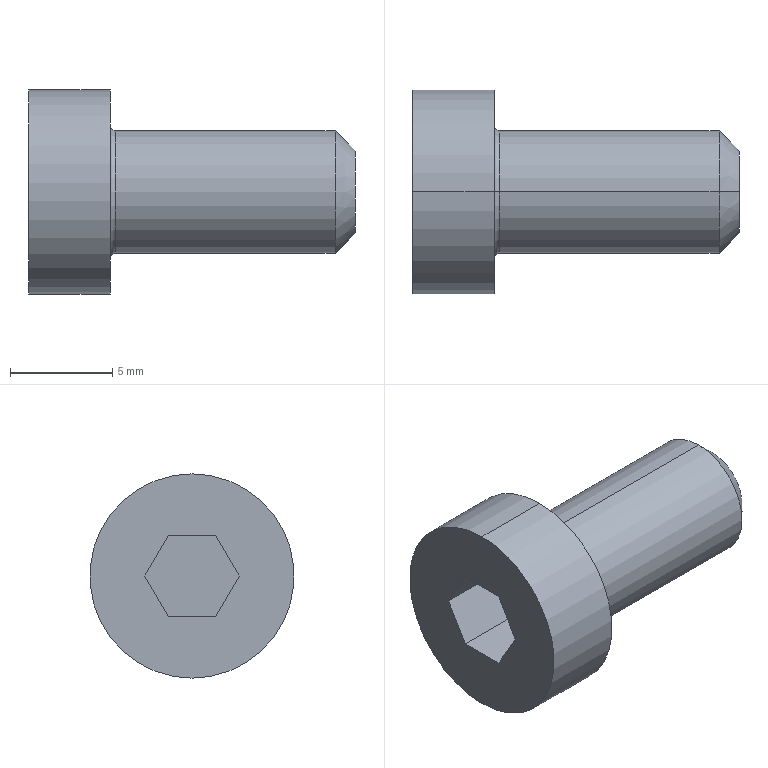Part | STEP file | CBSSTH6-12-24 | 1 solid | 18 faces | box 16 x 10 x 10 mm | volume 603.762 mm3 | plane 10 | cylinder 4 | torus 2 | cone 2 | commonest cylinder face diameters 6 x2 10 x2
STEP:
#1=CARTESIAN_POINT('',(0.,0.,0.));
#2=DIRECTION('',(0.,0.,1.));
#3=DIRECTION('',(1.,0.,0.));
#4=AXIS2_PLACEMENT_3D('',#1,#2,#3);
#5=CARTESIAN_POINT('',(0.,0.,5.));
#6=VERTEX_POINT('',#5);
#7=CARTESIAN_POINT('',(0.,0.,-5.));
#8=VERTEX_POINT('',#7);
#9=CARTESIAN_POINT('',(0.,0.,0.));
#10=DIRECTION('',(-1.,0.,0.));
#11=DIRECTION('',(0.,0.,1.));
#12=AXIS2_PLACEMENT_3D('',#9,#10,#11);
#13=CIRCLE('',#12,5.);
#14=CARTESIAN_POINT('',(-4.8,0.,0.));
#15=DIRECTION('',(-1.,0.,0.));
#16=DIRECTION('',(0.,0.,1.));
#17=AXIS2_PLACEMENT_3D('',#14,#15,#16);
#18=CYLINDRICAL_SURFACE('',#17,5.);
#19=CARTESIAN_POINT('',(0.,-4.8));
#20=DIRECTION('',(1.,0.));
#21=VECTOR('',#20,1.);
#22=LINE('',#19,#21);
#23=(GEOMETRIC_REPRESENTATION_CONTEXT(2)PARAMETRIC_REPRESENTATION_CONTEXT()REPRESENTATION_CONTEXT('',''));
#24=DEFINITIONAL_REPRESENTATION('',(#22),#23);
#25=PCURVE('',#18,#24);
#26=CARTESIAN_POINT('',(0.,-3.25,0.));
#27=DIRECTION('',(1.,0.,0.));
#28=DIRECTION('',(0.,0.,-1.));
#29=AXIS2_PLACEMENT_3D('',#26,#27,#28);
#30=PLANE('',#29);
#31=CARTESIAN_POINT('',(-5.,3.25));
#32=CARTESIAN_POINT('',(-5.,11.91));
#33=CARTESIAN_POINT('',(2.5,7.58));
#34=CARTESIAN_POINT('',(10.,3.25));
#35=CARTESIAN_POINT('',(2.5,-1.08));
#36=CARTESIAN_POINT('',(-5.,-5.41));
#37=CARTESIAN_POINT('',(-5.,3.25));
#38=(BOUNDED_CURVE()B_SPLINE_CURVE(2,(#31,#32,#33,#34,#35,#36,#37),.UNSPECIFIED.,.T.,.F.)B_SPLINE_CURVE_WITH_KNOTS((1,2,2,2,2,1),(-2.094,0.,2.094,4.189,6.283,8.378),.UNSPECIFIED.)CURVE()GEOMETRIC_REPRESENTATION_ITEM()RATIONAL_B_SPLINE_CURVE((1.,0.5,1.,0.5,1.,0.5,1.))REPRESENTATION_ITEM(''));
#39=(GEOMETRIC_REPRESENTATION_CONTEXT(2)PARAMETRIC_REPRESENTATION_CONTEXT()REPRESENTATION_CONTEXT('',''));
#40=DEFINITIONAL_REPRESENTATION('',(#38),#39);
#41=PCURVE('',#30,#40);
#42=SURFACE_CURVE('',#13,(#25,#41),.PCURVE_S1.);
#43=EDGE_CURVE('',#6,#8,#42,.T.);
#44=ORIENTED_EDGE('',*,*,#43,.T.);
#45=CARTESIAN_POINT('',(-4.,0.,-5.));
#46=VERTEX_POINT('',#45);
#47=CARTESIAN_POINT('',(-4.8,0.,-5.));
#48=DIRECTION('',(-1.,0.,0.));
#49=VECTOR('',#48,1.);
#50=LINE('',#47,#49);
#51=CARTESIAN_POINT('',(3.142,0.));
#52=DIRECTION('',(0.,1.));
#53=VECTOR('',#52,1.);
#54=LINE('',#51,#53);
#55=(GEOMETRIC_REPRESENTATION_CONTEXT(2)PARAMETRIC_REPRESENTATION_CONTEXT()REPRESENTATION_CONTEXT('',''));
#56=DEFINITIONAL_REPRESENTATION('',(#54),#55);
#57=PCURVE('',#18,#56);
#58=CARTESIAN_POINT('',(-4.8,0.,0.));
#59=DIRECTION('',(-1.,0.,0.));
#60=DIRECTION('',(0.,0.,1.));
#61=AXIS2_PLACEMENT_3D('',#58,#59,#60);
#62=CYLINDRICAL_SURFACE('',#61,5.);
#63=CARTESIAN_POINT('',(3.142,0.));
#64=DIRECTION('',(0.,1.));
#65=VECTOR('',#64,1.);
#66=LINE('',#63,#65);
#67=(GEOMETRIC_REPRESENTATION_CONTEXT(2)PARAMETRIC_REPRESENTATION_CONTEXT()REPRESENTATION_CONTEXT('',''));
#68=DEFINITIONAL_REPRESENTATION('',(#66),#67);
#69=PCURVE('',#62,#68);
#70=SURFACE_CURVE('',#50,(#57,#69),.PCURVE_S1.);
#71=EDGE_CURVE('',#8,#46,#70,.T.);
#72=ORIENTED_EDGE('',*,*,#71,.T.);
#73=CARTESIAN_POINT('',(-4.,0.,5.));
#74=VERTEX_POINT('',#73);
#75=CARTESIAN_POINT('',(-4.,0.,0.));
#76=DIRECTION('',(-1.,0.,0.));
#77=DIRECTION('',(0.,0.,1.));
#78=AXIS2_PLACEMENT_3D('',#75,#76,#77);
#79=CIRCLE('',#78,5.);
#80=CARTESIAN_POINT('',(0.,-0.8));
#81=DIRECTION('',(1.,0.));
#82=VECTOR('',#81,1.);
#83=LINE('',#80,#82);
#84=(GEOMETRIC_REPRESENTATION_CONTEXT(2)PARAMETRIC_REPRESENTATION_CONTEXT()REPRESENTATION_CONTEXT('',''));
#85=DEFINITIONAL_REPRESENTATION('',(#83),#84);
#86=PCURVE('',#18,#85);
#87=CARTESIAN_POINT('',(-4.,-5.,0.));
#88=DIRECTION('',(-1.,0.,0.));
#89=DIRECTION('',(0.,0.,1.));
#90=AXIS2_PLACEMENT_3D('',#87,#88,#89);
#91=PLANE('',#90);
#92=CARTESIAN_POINT('',(0.,5.));
#93=DIRECTION('',(1.,0.));
#94=AXIS2_PLACEMENT_2D('',#92,#93);
#95=CIRCLE('',#94,5.);
#96=(GEOMETRIC_REPRESENTATION_CONTEXT(2)PARAMETRIC_REPRESENTATION_CONTEXT()REPRESENTATION_CONTEXT('',''));
#97=DEFINITIONAL_REPRESENTATION('',(#95),#96);
#98=PCURVE('',#91,#97);
#99=SURFACE_CURVE('',#79,(#86,#98),.PCURVE_S1.);
#100=EDGE_CURVE('',#74,#46,#99,.T.);
#101=ORIENTED_EDGE('',*,*,#100,.F.);
#102=CARTESIAN_POINT('',(-4.8,0.,5.));
#103=DIRECTION('',(-1.,0.,0.));
#104=VECTOR('',#103,1.);
#105=LINE('',#102,#104);
#106=CARTESIAN_POINT('',(0.,0.));
#107=DIRECTION('',(0.,1.));
#108=VECTOR('',#107,1.);
#109=LINE('',#106,#108);
#110=(GEOMETRIC_REPRESENTATION_CONTEXT(2)PARAMETRIC_REPRESENTATION_CONTEXT()REPRESENTATION_CONTEXT('',''));
#111=DEFINITIONAL_REPRESENTATION('',(#109),#110);
#112=PCURVE('',#18,#111);
#113=CARTESIAN_POINT('',(6.283,0.));
#114=DIRECTION('',(0.,1.));
#115=VECTOR('',#114,1.);
#116=LINE('',#113,#115);
#117=(GEOMETRIC_REPRESENTATION_CONTEXT(2)PARAMETRIC_REPRESENTATION_CONTEXT()REPRESENTATION_CONTEXT('',''));
#118=DEFINITIONAL_REPRESENTATION('',(#116),#117);
#119=PCURVE('',#62,#118);
#120=SURFACE_CURVE('',#105,(#112,#119),.PCURVE_S1.);
#121=EDGE_CURVE('',#6,#74,#120,.T.);
#122=ORIENTED_EDGE('',*,*,#121,.F.);
#123=EDGE_LOOP('',(#44,#72,#101,#122));
#124=FACE_BOUND('',#123,.T.);
#125=ADVANCED_FACE('',(#124),#18,.T.);
#126=CARTESIAN_POINT('',(0.,0.,3.25));
#127=VERTEX_POINT('',#126);
#128=CARTESIAN_POINT('',(0.25,0.,3.));
#129=VERTEX_POINT('',#128);
#130=CARTESIAN_POINT('',(0.25,0.,3.25));
#131=DIRECTION('',(0.,-1.,0.));
#132=DIRECTION('',(0.,0.,-1.));
#133=AXIS2_PLACEMENT_3D('',#130,#131,#132);
#134=CIRCLE('',#133,0.25);
#135=CARTESIAN_POINT('',(0.25,0.,0.));
#136=DIRECTION('',(-1.,0.,0.));
#137=DIRECTION('',(0.,0.,1.));
#138=AXIS2_PLACEMENT_3D('',#135,#136,#137);
#139=TOROIDAL_SURFACE('',#138,3.25,0.25);
#140=CARTESIAN_POINT('',(6.283,-3.142));
#141=DIRECTION('',(0.,1.));
#142=VECTOR('',#141,1.);
#143=LINE('',#140,#142);
#144=(GEOMETRIC_REPRESENTATION_CONTEXT(2)PARAMETRIC_REPRESENTATION_CONTEXT()REPRESENTATION_CONTEXT('',''));
#145=DEFINITIONAL_REPRESENTATION('',(#143),#144);
#146=PCURVE('',#139,#145);
#147=CARTESIAN_POINT('',(0.25,0.,0.));
#148=DIRECTION('',(-1.,0.,0.));
#149=DIRECTION('',(0.,0.,1.));
#150=AXIS2_PLACEMENT_3D('',#147,#148,#149);
#151=TOROIDAL_SURFACE('',#150,3.25,0.25);
#152=CARTESIAN_POINT('',(0.,-3.142));
#153=DIRECTION('',(0.,1.));
#154=VECTOR('',#153,1.);
#155=LINE('',#152,#154);
#156=(GEOMETRIC_REPRESENTATION_CONTEXT(2)PARAMETRIC_REPRESENTATION_CONTEXT()REPRESENTATION_CONTEXT('',''));
#157=DEFINITIONAL_REPRESENTATION('',(#155),#156);
#158=PCURVE('',#151,#157);
#159=SURFACE_CURVE('',#134,(#146,#158),.PCURVE_S1.);
#160=EDGE_CURVE('',#127,#129,#159,.T.);
#161=ORIENTED_EDGE('',*,*,#160,.T.);
#162=CARTESIAN_POINT('',(0.25,0.,-3.));
#163=VERTEX_POINT('',#162);
#164=CARTESIAN_POINT('',(0.25,0.,0.));
#165=DIRECTION('',(-1.,0.,0.));
#166=DIRECTION('',(0.,0.,1.));
#167=AXIS2_PLACEMENT_3D('',#164,#165,#166);
#168=CIRCLE('',#167,3.);
#169=CARTESIAN_POINT('',(0.,3.142));
#170=DIRECTION('',(1.,0.));
#171=VECTOR('',#170,1.);
#172=LINE('',#169,#171);
#173=(GEOMETRIC_REPRESENTATION_CONTEXT(2)PARAMETRIC_REPRESENTATION_CONTEXT()REPRESENTATION_CONTEXT('',''));
#174=DEFINITIONAL_REPRESENTATION('',(#172),#173);
#175=PCURVE('',#139,#174);
#176=CARTESIAN_POINT('',(-4.8,0.,0.));
#177=DIRECTION('',(-1.,0.,0.));
#178=DIRECTION('',(0.,0.,1.));
#179=AXIS2_PLACEMENT_3D('',#176,#177,#178);
#180=CYLINDRICAL_SURFACE('',#179,3.);
#181=CARTESIAN_POINT('',(0.,-5.05));
#182=DIRECTION('',(1.,0.));
#183=VECTOR('',#182,1.);
#184=LINE('',#181,#183);
#185=(GEOMETRIC_REPRESENTATION_CONTEXT(2)PARAMETRIC_REPRESENTATION_CONTEXT()REPRESENTATION_CONTEXT('',''));
#186=DEFINITIONAL_REPRESENTATION('',(#184),#185);
#187=PCURVE('',#180,#186);
#188=SURFACE_CURVE('',#168,(#175,#187),.PCURVE_S1.);
#189=EDGE_CURVE('',#163,#129,#188,.T.);
#190=ORIENTED_EDGE('',*,*,#189,.F.);
#191=CARTESIAN_POINT('',(0.,0.,-3.25));
#192=VERTEX_POINT('',#191);
#193=CARTESIAN_POINT('',(0.25,0.,-3.25));
#194=DIRECTION('',(0.,1.,0.));
#195=DIRECTION('',(0.,0.,1.));
#196=AXIS2_PLACEMENT_3D('',#193,#194,#195);
#197=CIRCLE('',#196,0.25);
#198=CARTESIAN_POINT('',(3.142,-3.142));
#199=DIRECTION('',(0.,1.));
#200=VECTOR('',#199,1.);
#201=LINE('',#198,#200);
#202=(GEOMETRIC_REPRESENTATION_CONTEXT(2)PARAMETRIC_REPRESENTATION_CONTEXT()REPRESENTATION_CONTEXT('',''));
#203=DEFINITIONAL_REPRESENTATION('',(#201),#202);
#204=PCURVE('',#139,#203);
#205=CARTESIAN_POINT('',(3.142,-3.142));
#206=DIRECTION('',(0.,1.));
#207=VECTOR('',#206,1.);
#208=LINE('',#205,#207);
#209=(GEOMETRIC_REPRESENTATION_CONTEXT(2)PARAMETRIC_REPRESENTATION_CONTEXT()REPRESENTATION_CONTEXT('',''));
#210=DEFINITIONAL_REPRESENTATION('',(#208),#209);
#211=PCURVE('',#151,#210);
#212=SURFACE_CURVE('',#197,(#204,#211),.PCURVE_S1.);
#213=EDGE_CURVE('',#192,#163,#212,.T.);
#214=ORIENTED_EDGE('',*,*,#213,.F.);
#215=CARTESIAN_POINT('',(0.,0.,0.));
#216=DIRECTION('',(-1.,0.,0.));
#217=DIRECTION('',(0.,0.,1.));
#218=AXIS2_PLACEMENT_3D('',#215,#216,#217);
#219=CIRCLE('',#218,3.25);
#220=CARTESIAN_POINT('',(0.,1.571));
#221=DIRECTION('',(1.,0.));
#222=VECTOR('',#221,1.);
#223=LINE('',#220,#222);
#224=(GEOMETRIC_REPRESENTATION_CONTEXT(2)PARAMETRIC_REPRESENTATION_CONTEXT()REPRESENTATION_CONTEXT('',''));
#225=DEFINITIONAL_REPRESENTATION('',(#223),#224);
#226=PCURVE('',#139,#225);
#227=CARTESIAN_POINT('',(-3.25,3.25));
#228=CARTESIAN_POINT('',(-3.25,8.879));
#229=CARTESIAN_POINT('',(1.625,6.065));
#230=CARTESIAN_POINT('',(6.5,3.25));
#231=CARTESIAN_POINT('',(1.625,0.4354));
#232=CARTESIAN_POINT('',(-3.25,-2.379));
#233=CARTESIAN_POINT('',(-3.25,3.25));
#234=(BOUNDED_CURVE()B_SPLINE_CURVE(2,(#227,#228,#229,#230,#231,#232,#233),.UNSPECIFIED.,.T.,.F.)B_SPLINE_CURVE_WITH_KNOTS((1,2,2,2,2,1),(-2.094,0.,2.094,4.189,6.283,8.378),.UNSPECIFIED.)CURVE()GEOMETRIC_REPRESENTATION_ITEM()RATIONAL_B_SPLINE_CURVE((1.,0.5,1.,0.5,1.,0.5,1.))REPRESENTATION_ITEM(''));
#235=(GEOMETRIC_REPRESENTATION_CONTEXT(2)PARAMETRIC_REPRESENTATION_CONTEXT()REPRESENTATION_CONTEXT('',''));
#236=DEFINITIONAL_REPRESENTATION('',(#234),#235);
#237=PCURVE('',#30,#236);
#238=SURFACE_CURVE('',#219,(#226,#237),.PCURVE_S1.);
#239=EDGE_CURVE('',#192,#127,#238,.T.);
#240=ORIENTED_EDGE('',*,*,#239,.T.);
#241=EDGE_LOOP('',(#161,#190,#214,#240));
#242=FACE_BOUND('',#241,.F.);
#243=ADVANCED_FACE('',(#242),#139,.F.);
#244=CARTESIAN_POINT('',(11.,0.,3.));
#245=VERTEX_POINT('',#244);
#246=CARTESIAN_POINT('',(11.,0.,-3.));
#247=VERTEX_POINT('',#246);
#248=CARTESIAN_POINT('',(11.,0.,0.));
#249=DIRECTION('',(-1.,0.,0.));
#250=DIRECTION('',(0.,0.,1.));
#251=AXIS2_PLACEMENT_3D('',#248,#249,#250);
#252=CIRCLE('',#251,3.);
#253=CARTESIAN_POINT('',(-4.8,0.,0.));
#254=DIRECTION('',(-1.,0.,0.));
#255=DIRECTION('',(0.,0.,1.));
#256=AXIS2_PLACEMENT_3D('',#253,#254,#255);
#257=CYLINDRICAL_SURFACE('',#256,3.);
#258=CARTESIAN_POINT('',(0.,-15.8));
#259=DIRECTION('',(1.,0.));
#260=VECTOR('',#259,1.);
#261=LINE('',#258,#260);
#262=(GEOMETRIC_REPRESENTATION_CONTEXT(2)PARAMETRIC_REPRESENTATION_CONTEXT()REPRESENTATION_CONTEXT('',''));
#263=DEFINITIONAL_REPRESENTATION('',(#261),#262);
#264=PCURVE('',#257,#263);
#265=CARTESIAN_POINT('',(11.,0.,0.));
#266=DIRECTION('',(-1.,0.,0.));
#267=DIRECTION('',(0.,0.,1.));
#268=AXIS2_PLACEMENT_3D('',#265,#266,#267);
#269=CONICAL_SURFACE('',#268,3.,0.7854);
#270=CARTESIAN_POINT('',(0.,0.));
#271=DIRECTION('',(1.,0.));
#272=VECTOR('',#271,1.);
#273=LINE('',#270,#272);
#274=(GEOMETRIC_REPRESENTATION_CONTEXT(2)PARAMETRIC_REPRESENTATION_CONTEXT()REPRESENTATION_CONTEXT('',''));
#275=DEFINITIONAL_REPRESENTATION('',(#273),#274);
#276=PCURVE('',#269,#275);
#277=SURFACE_CURVE('',#252,(#264,#276),.PCURVE_S1.);
#278=EDGE_CURVE('',#245,#247,#277,.T.);
#279=ORIENTED_EDGE('',*,*,#278,.T.);
#280=CARTESIAN_POINT('',(-4.8,0.,-3.));
#281=DIRECTION('',(-1.,0.,0.));
#282=VECTOR('',#281,1.);
#283=LINE('',#280,#282);
#284=CARTESIAN_POINT('',(3.142,0.));
#285=DIRECTION('',(0.,1.));
#286=VECTOR('',#285,1.);
#287=LINE('',#284,#286);
#288=(GEOMETRIC_REPRESENTATION_CONTEXT(2)PARAMETRIC_REPRESENTATION_CONTEXT()REPRESENTATION_CONTEXT('',''));
#289=DEFINITIONAL_REPRESENTATION('',(#287),#288);
#290=PCURVE('',#257,#289);
#291=CARTESIAN_POINT('',(3.142,0.));
#292=DIRECTION('',(0.,1.));
#293=VECTOR('',#292,1.);
#294=LINE('',#291,#293);
#295=(GEOMETRIC_REPRESENTATION_CONTEXT(2)PARAMETRIC_REPRESENTATION_CONTEXT()REPRESENTATION_CONTEXT('',''));
#296=DEFINITIONAL_REPRESENTATION('',(#294),#295);
#297=PCURVE('',#180,#296);
#298=SURFACE_CURVE('',#283,(#290,#297),.PCURVE_S1.);
#299=EDGE_CURVE('',#247,#163,#298,.T.);
#300=ORIENTED_EDGE('',*,*,#299,.T.);
#301=CARTESIAN_POINT('',(0.25,0.,0.));
#302=DIRECTION('',(-1.,0.,0.));
#303=DIRECTION('',(0.,0.,1.));
#304=AXIS2_PLACEMENT_3D('',#301,#302,#303);
#305=CIRCLE('',#304,3.);
#306=CARTESIAN_POINT('',(0.,-5.05));
#307=DIRECTION('',(1.,0.));
#308=VECTOR('',#307,1.);
#309=LINE('',#306,#308);
#310=(GEOMETRIC_REPRESENTATION_CONTEXT(2)PARAMETRIC_REPRESENTATION_CONTEXT()REPRESENTATION_CONTEXT('',''));
#311=DEFINITIONAL_REPRESENTATION('',(#309),#310);
#312=PCURVE('',#257,#311);
#313=CARTESIAN_POINT('',(0.,3.142));
#314=DIRECTION('',(1.,0.));
#315=VECTOR('',#314,1.);
#316=LINE('',#313,#315);
#317=(GEOMETRIC_REPRESENTATION_CONTEXT(2)PARAMETRIC_REPRESENTATION_CONTEXT()REPRESENTATION_CONTEXT('',''));
#318=DEFINITIONAL_REPRESENTATION('',(#316),#317);
#319=PCURVE('',#151,#318);
#320=SURFACE_CURVE('',#305,(#312,#319),.PCURVE_S1.);
#321=EDGE_CURVE('',#129,#163,#320,.T.);
#322=ORIENTED_EDGE('',*,*,#321,.F.);
#323=CARTESIAN_POINT('',(-4.8,0.,3.));
#324=DIRECTION('',(-1.,0.,0.));
#325=VECTOR('',#324,1.);
#326=LINE('',#323,#325);
#327=CARTESIAN_POINT('',(0.,0.));
#328=DIRECTION('',(0.,1.));
#329=VECTOR('',#328,1.);
#330=LINE('',#327,#329);
#331=(GEOMETRIC_REPRESENTATION_CONTEXT(2)PARAMETRIC_REPRESENTATION_CONTEXT()REPRESENTATION_CONTEXT('',''));
#332=DEFINITIONAL_REPRESENTATION('',(#330),#331);
#333=PCURVE('',#257,#332);
#334=CARTESIAN_POINT('',(6.283,0.));
#335=DIRECTION('',(0.,1.));
#336=VECTOR('',#335,1.);
#337=LINE('',#334,#336);
#338=(GEOMETRIC_REPRESENTATION_CONTEXT(2)PARAMETRIC_REPRESENTATION_CONTEXT()REPRESENTATION_CONTEXT('',''));
#339=DEFINITIONAL_REPRESENTATION('',(#337),#338);
#340=PCURVE('',#180,#339);
#341=SURFACE_CURVE('',#326,(#333,#340),.PCURVE_S1.);
#342=EDGE_CURVE('',#245,#129,#341,.T.);
#343=ORIENTED_EDGE('',*,*,#342,.F.);
#344=EDGE_LOOP('',(#279,#300,#322,#343));
#345=FACE_BOUND('',#344,.T.);
#346=ADVANCED_FACE('',(#345),#257,.T.);
#347=CARTESIAN_POINT('',(12.,0.,2.));
#348=VERTEX_POINT('',#347);
#349=CARTESIAN_POINT('',(12.,0.,-2.));
#350=VERTEX_POINT('',#349);
#351=CARTESIAN_POINT('',(12.,0.,0.));
#352=DIRECTION('',(-1.,0.,0.));
#353=DIRECTION('',(0.,0.,1.));
#354=AXIS2_PLACEMENT_3D('',#351,#352,#353);
#355=CIRCLE('',#354,2.);
#356=CARTESIAN_POINT('',(0.,-1.));
#357=DIRECTION('',(1.,0.));
#358=VECTOR('',#357,1.);
#359=LINE('',#356,#358);
#360=(GEOMETRIC_REPRESENTATION_CONTEXT(2)PARAMETRIC_REPRESENTATION_CONTEXT()REPRESENTATION_CONTEXT('',''));
#361=DEFINITIONAL_REPRESENTATION('',(#359),#360);
#362=PCURVE('',#269,#361);
#363=CARTESIAN_POINT('',(12.,0.,0.));
#364=DIRECTION('',(1.,0.,0.));
#365=DIRECTION('',(0.,0.,-1.));
#366=AXIS2_PLACEMENT_3D('',#363,#364,#365);
#367=PLANE('',#366);
#368=CARTESIAN_POINT('',(-2.,0.));
#369=CARTESIAN_POINT('',(-2.,3.464));
#370=CARTESIAN_POINT('',(1.,1.732));
#371=CARTESIAN_POINT('',(4.,0.));
#372=CARTESIAN_POINT('',(1.,-1.732));
#373=CARTESIAN_POINT('',(-2.,-3.464));
#374=CARTESIAN_POINT('',(-2.,0.));
#375=(BOUNDED_CURVE()B_SPLINE_CURVE(2,(#368,#369,#370,#371,#372,#373,#374),.UNSPECIFIED.,.T.,.F.)B_SPLINE_CURVE_WITH_KNOTS((1,2,2,2,2,1),(-2.094,0.,2.094,4.189,6.283,8.378),.UNSPECIFIED.)CURVE()GEOMETRIC_REPRESENTATION_ITEM()RATIONAL_B_SPLINE_CURVE((1.,0.5,1.,0.5,1.,0.5,1.))REPRESENTATION_ITEM(''));
#376=(GEOMETRIC_REPRESENTATION_CONTEXT(2)PARAMETRIC_REPRESENTATION_CONTEXT()REPRESENTATION_CONTEXT('',''));
#377=DEFINITIONAL_REPRESENTATION('',(#375),#376);
#378=PCURVE('',#367,#377);
#379=SURFACE_CURVE('',#355,(#362,#378),.PCURVE_S1.);
#380=EDGE_CURVE('',#348,#350,#379,.T.);
#381=ORIENTED_EDGE('',*,*,#380,.T.);
#382=CARTESIAN_POINT('',(11.,0.,-3.));
#383=DIRECTION('',(-0.7071,0.,-0.7071));
#384=VECTOR('',#383,1.);
#385=LINE('',#382,#384);
#386=CARTESIAN_POINT('',(3.142,0.));
#387=DIRECTION('',(0.,1.));
#388=VECTOR('',#387,1.);
#389=LINE('',#386,#388);
#390=(GEOMETRIC_REPRESENTATION_CONTEXT(2)PARAMETRIC_REPRESENTATION_CONTEXT()REPRESENTATION_CONTEXT('',''));
#391=DEFINITIONAL_REPRESENTATION('',(#389),#390);
#392=PCURVE('',#269,#391);
#393=CARTESIAN_POINT('',(11.,0.,0.));
#394=DIRECTION('',(-1.,0.,0.));
#395=DIRECTION('',(0.,0.,1.));
#396=AXIS2_PLACEMENT_3D('',#393,#394,#395);
#397=CONICAL_SURFACE('',#396,3.,0.7854);
#398=CARTESIAN_POINT('',(3.142,0.));
#399=DIRECTION('',(0.,1.));
#400=VECTOR('',#399,1.);
#401=LINE('',#398,#400);
#402=(GEOMETRIC_REPRESENTATION_CONTEXT(2)PARAMETRIC_REPRESENTATION_CONTEXT()REPRESENTATION_CONTEXT('',''));
#403=DEFINITIONAL_REPRESENTATION('',(#401),#402);
#404=PCURVE('',#397,#403);
#405=SURFACE_CURVE('',#385,(#392,#404),.PCURVE_S1.);
#406=EDGE_CURVE('',#350,#247,#405,.T.);
#407=ORIENTED_EDGE('',*,*,#406,.T.);
#408=ORIENTED_EDGE('',*,*,#278,.F.);
#409=CARTESIAN_POINT('',(11.,0.,3.));
#410=DIRECTION('',(-0.7071,0.,0.7071));
#411=VECTOR('',#410,1.);
#412=LINE('',#409,#411);
#413=CARTESIAN_POINT('',(0.,0.));
#414=DIRECTION('',(0.,1.));
#415=VECTOR('',#414,1.);
#416=LINE('',#413,#415);
#417=(GEOMETRIC_REPRESENTATION_CONTEXT(2)PARAMETRIC_REPRESENTATION_CONTEXT()REPRESENTATION_CONTEXT('',''));
#418=DEFINITIONAL_REPRESENTATION('',(#416),#417);
#419=PCURVE('',#269,#418);
#420=CARTESIAN_POINT('',(6.283,0.));
#421=DIRECTION('',(0.,1.));
#422=VECTOR('',#421,1.);
#423=LINE('',#420,#422);
#424=(GEOMETRIC_REPRESENTATION_CONTEXT(2)PARAMETRIC_REPRESENTATION_CONTEXT()REPRESENTATION_CONTEXT('',''));
#425=DEFINITIONAL_REPRESENTATION('',(#423),#424);
#426=PCURVE('',#397,#425);
#427=SURFACE_CURVE('',#412,(#419,#426),.PCURVE_S1.);
#428=EDGE_CURVE('',#348,#245,#427,.T.);
#429=ORIENTED_EDGE('',*,*,#428,.F.);
#430=EDGE_LOOP('',(#381,#407,#408,#429));
#431=FACE_BOUND('',#430,.T.);
#432=ADVANCED_FACE('',(#431),#269,.T.);
#433=CARTESIAN_POINT('',(-4.,1.155,2.));
#434=VERTEX_POINT('',#433);
#435=CARTESIAN_POINT('',(-4.,2.309,0.));
#436=VERTEX_POINT('',#435);
#437=CARTESIAN_POINT('',(-4.,1.155,2.));
#438=DIRECTION('',(0.,0.5,-0.866));
#439=VECTOR('',#438,1.);
#440=LINE('',#437,#439);
#441=CARTESIAN_POINT('',(2.,6.155));
#442=DIRECTION('',(-0.866,0.5));
#443=VECTOR('',#442,1.);
#444=LINE('',#441,#443);
#445=(GEOMETRIC_REPRESENTATION_CONTEXT(2)PARAMETRIC_REPRESENTATION_CONTEXT()REPRESENTATION_CONTEXT('',''));
#446=DEFINITIONAL_REPRESENTATION('',(#444),#445);
#447=PCURVE('',#91,#446);
#448=CARTESIAN_POINT('',(-1.,1.155,2.));
#449=DIRECTION('',(0.,0.866,0.5));
#450=DIRECTION('',(0.,-0.5,0.866));
#451=AXIS2_PLACEMENT_3D('',#448,#449,#450);
#452=PLANE('',#451);
#453=CARTESIAN_POINT('',(0.,-3.));
#454=DIRECTION('',(-1.,0.));
#455=VECTOR('',#454,1.);
#456=LINE('',#453,#455);
#457=(GEOMETRIC_REPRESENTATION_CONTEXT(2)PARAMETRIC_REPRESENTATION_CONTEXT()REPRESENTATION_CONTEXT('',''));
#458=DEFINITIONAL_REPRESENTATION('',(#456),#457);
#459=PCURVE('',#452,#458);
#460=SURFACE_CURVE('',#440,(#447,#459),.PCURVE_S1.);
#461=EDGE_CURVE('',#434,#436,#460,.T.);
#462=ORIENTED_EDGE('',*,*,#461,.F.);
#463=CARTESIAN_POINT('',(-4.,-1.155,2.));
#464=VERTEX_POINT('',#463);
#465=CARTESIAN_POINT('',(-4.,-1.155,2.));
#466=DIRECTION('',(0.,1.,0.));
#467=VECTOR('',#466,1.);
#468=LINE('',#465,#467);
#469=CARTESIAN_POINT('',(2.,3.845));
#470=DIRECTION('',(0.,1.));
#471=VECTOR('',#470,1.);
#472=LINE('',#469,#471);
#473=(GEOMETRIC_REPRESENTATION_CONTEXT(2)PARAMETRIC_REPRESENTATION_CONTEXT()REPRESENTATION_CONTEXT('',''));
#474=DEFINITIONAL_REPRESENTATION('',(#472),#473);
#475=PCURVE('',#91,#474);
#476=CARTESIAN_POINT('',(-1.,-1.155,2.));
#477=DIRECTION('',(0.,0.,1.));
#478=DIRECTION('',(1.,0.,0.));
#479=AXIS2_PLACEMENT_3D('',#476,#477,#478);
#480=PLANE('',#479);
#481=CARTESIAN_POINT('',(-3.,0.));
#482=DIRECTION('',(0.,1.));
#483=VECTOR('',#482,1.);
#484=LINE('',#481,#483);
#485=(GEOMETRIC_REPRESENTATION_CONTEXT(2)PARAMETRIC_REPRESENTATION_CONTEXT()REPRESENTATION_CONTEXT('',''));
#486=DEFINITIONAL_REPRESENTATION('',(#484),#485);
#487=PCURVE('',#480,#486);
#488=SURFACE_CURVE('',#468,(#475,#487),.PCURVE_S1.);
#489=EDGE_CURVE('',#464,#434,#488,.T.);
#490=ORIENTED_EDGE('',*,*,#489,.F.);
#491=CARTESIAN_POINT('',(-4.,-2.309,0.));
#492=VERTEX_POINT('',#491);
#493=CARTESIAN_POINT('',(-4.,-2.309,0.));
#494=DIRECTION('',(0.,0.5,0.866));
#495=VECTOR('',#494,1.);
#496=LINE('',#493,#495);
#497=CARTESIAN_POINT('',(0.,2.691));
#498=DIRECTION('',(0.866,0.5));
#499=VECTOR('',#498,1.);
#500=LINE('',#497,#499);
#501=(GEOMETRIC_REPRESENTATION_CONTEXT(2)PARAMETRIC_REPRESENTATION_CONTEXT()REPRESENTATION_CONTEXT('',''));
#502=DEFINITIONAL_REPRESENTATION('',(#500),#501);
#503=PCURVE('',#91,#502);
#504=CARTESIAN_POINT('',(-1.,-2.309,0.));
#505=DIRECTION('',(0.,-0.866,0.5));
#506=DIRECTION('',(0.,-0.5,-0.866));
#507=AXIS2_PLACEMENT_3D('',#504,#505,#506);
#508=PLANE('',#507);
#509=CARTESIAN_POINT('',(0.,-3.));
#510=DIRECTION('',(-1.,0.));
#511=VECTOR('',#510,1.);
#512=LINE('',#509,#511);
#513=(GEOMETRIC_REPRESENTATION_CONTEXT(2)PARAMETRIC_REPRESENTATION_CONTEXT()REPRESENTATION_CONTEXT('',''));
#514=DEFINITIONAL_REPRESENTATION('',(#512),#513);
#515=PCURVE('',#508,#514);
#516=SURFACE_CURVE('',#496,(#503,#515),.PCURVE_S1.);
#517=EDGE_CURVE('',#492,#464,#516,.T.);
#518=ORIENTED_EDGE('',*,*,#517,.F.);
#519=CARTESIAN_POINT('',(-4.,-1.155,-2.));
#520=VERTEX_POINT('',#519);
#521=CARTESIAN_POINT('',(-4.,-1.155,-2.));
#522=DIRECTION('',(0.,-0.5,0.866));
#523=VECTOR('',#522,1.);
#524=LINE('',#521,#523);
#525=CARTESIAN_POINT('',(-2.,3.845));
#526=DIRECTION('',(0.866,-0.5));
#527=VECTOR('',#526,1.);
#528=LINE('',#525,#527);
#529=(GEOMETRIC_REPRESENTATION_CONTEXT(2)PARAMETRIC_REPRESENTATION_CONTEXT()REPRESENTATION_CONTEXT('',''));
#530=DEFINITIONAL_REPRESENTATION('',(#528),#529);
#531=PCURVE('',#91,#530);
#532=CARTESIAN_POINT('',(-1.,-1.155,-2.));
#533=DIRECTION('',(0.,-0.866,-0.5));
#534=DIRECTION('',(0.,0.5,-0.866));
#535=AXIS2_PLACEMENT_3D('',#532,#533,#534);
#536=PLANE('',#535);
#537=CARTESIAN_POINT('',(0.,-3.));
#538=DIRECTION('',(-1.,0.));
#539=VECTOR('',#538,1.);
#540=LINE('',#537,#539);
#541=(GEOMETRIC_REPRESENTATION_CONTEXT(2)PARAMETRIC_REPRESENTATION_CONTEXT()REPRESENTATION_CONTEXT('',''));
#542=DEFINITIONAL_REPRESENTATION('',(#540),#541);
#543=PCURVE('',#536,#542);
#544=SURFACE_CURVE('',#524,(#531,#543),.PCURVE_S1.);
#545=EDGE_CURVE('',#520,#492,#544,.T.);
#546=ORIENTED_EDGE('',*,*,#545,.F.);
#547=CARTESIAN_POINT('',(-4.,1.155,-2.));
#548=VERTEX_POINT('',#547);
#549=CARTESIAN_POINT('',(-4.,1.155,-2.));
#550=DIRECTION('',(0.,-1.,0.));
#551=VECTOR('',#550,1.);
#552=LINE('',#549,#551);
#553=CARTESIAN_POINT('',(-2.,6.155));
#554=DIRECTION('',(0.,-1.));
#555=VECTOR('',#554,1.);
#556=LINE('',#553,#555);
#557=(GEOMETRIC_REPRESENTATION_CONTEXT(2)PARAMETRIC_REPRESENTATION_CONTEXT()REPRESENTATION_CONTEXT('',''));
#558=DEFINITIONAL_REPRESENTATION('',(#556),#557);
#559=PCURVE('',#91,#558);
#560=CARTESIAN_POINT('',(-1.,1.155,-2.));
#561=DIRECTION('',(0.,0.,-1.));
#562=DIRECTION('',(-1.,0.,0.));
#563=AXIS2_PLACEMENT_3D('',#560,#561,#562);
#564=PLANE('',#563);
#565=CARTESIAN_POINT('',(3.,0.));
#566=DIRECTION('',(0.,-1.));
#567=VECTOR('',#566,1.);
#568=LINE('',#565,#567);
#569=(GEOMETRIC_REPRESENTATION_CONTEXT(2)PARAMETRIC_REPRESENTATION_CONTEXT()REPRESENTATION_CONTEXT('',''));
#570=DEFINITIONAL_REPRESENTATION('',(#568),#569);
#571=PCURVE('',#564,#570);
#572=SURFACE_CURVE('',#552,(#559,#571),.PCURVE_S1.);
#573=EDGE_CURVE('',#548,#520,#572,.T.);
#574=ORIENTED_EDGE('',*,*,#573,.F.);
#575=CARTESIAN_POINT('',(-4.,2.309,0.));
#576=DIRECTION('',(0.,-0.5,-0.866));
#577=VECTOR('',#576,1.);
#578=LINE('',#575,#577);
#579=CARTESIAN_POINT('',(0.,7.309));
#580=DIRECTION('',(-0.866,-0.5));
#581=VECTOR('',#580,1.);
#582=LINE('',#579,#581);
#583=(GEOMETRIC_REPRESENTATION_CONTEXT(2)PARAMETRIC_REPRESENTATION_CONTEXT()REPRESENTATION_CONTEXT('',''));
#584=DEFINITIONAL_REPRESENTATION('',(#582),#583);
#585=PCURVE('',#91,#584);
#586=CARTESIAN_POINT('',(-1.,2.309,0.));
#587=DIRECTION('',(0.,0.866,-0.5));
#588=DIRECTION('',(0.,0.5,0.866));
#589=AXIS2_PLACEMENT_3D('',#586,#587,#588);
#590=PLANE('',#589);
#591=CARTESIAN_POINT('',(0.,-3.));
#592=DIRECTION('',(-1.,0.));
#593=VECTOR('',#592,1.);
#594=LINE('',#591,#593);
#595=(GEOMETRIC_REPRESENTATION_CONTEXT(2)PARAMETRIC_REPRESENTATION_CONTEXT()REPRESENTATION_CONTEXT('',''));
#596=DEFINITIONAL_REPRESENTATION('',(#594),#595);
#597=PCURVE('',#590,#596);
#598=SURFACE_CURVE('',#578,(#585,#597),.PCURVE_S1.);
#599=EDGE_CURVE('',#436,#548,#598,.T.);
#600=ORIENTED_EDGE('',*,*,#599,.F.);
#601=EDGE_LOOP('',(#462,#490,#518,#546,#574,#600));
#602=FACE_BOUND('',#601,.T.);
#603=ORIENTED_EDGE('',*,*,#100,.T.);
#604=CARTESIAN_POINT('',(-4.,0.,0.));
#605=DIRECTION('',(-1.,0.,0.));
#606=DIRECTION('',(0.,0.,1.));
#607=AXIS2_PLACEMENT_3D('',#604,#605,#606);
#608=CIRCLE('',#607,5.);
#609=CARTESIAN_POINT('',(0.,5.));
#610=DIRECTION('',(1.,0.));
#611=AXIS2_PLACEMENT_2D('',#609,#610);
#612=CIRCLE('',#611,5.);
#613=(GEOMETRIC_REPRESENTATION_CONTEXT(2)PARAMETRIC_REPRESENTATION_CONTEXT()REPRESENTATION_CONTEXT('',''));
#614=DEFINITIONAL_REPRESENTATION('',(#612),#613);
#615=PCURVE('',#91,#614);
#616=CARTESIAN_POINT('',(0.,-0.8));
#617=DIRECTION('',(1.,0.));
#618=VECTOR('',#617,1.);
#619=LINE('',#616,#618);
#620=(GEOMETRIC_REPRESENTATION_CONTEXT(2)PARAMETRIC_REPRESENTATION_CONTEXT()REPRESENTATION_CONTEXT('',''));
#621=DEFINITIONAL_REPRESENTATION('',(#619),#620);
#622=PCURVE('',#62,#621);
#623=SURFACE_CURVE('',#608,(#615,#622),.PCURVE_S1.);
#624=EDGE_CURVE('',#46,#74,#623,.T.);
#625=ORIENTED_EDGE('',*,*,#624,.T.);
#626=EDGE_LOOP('',(#603,#625));
#627=FACE_BOUND('',#626,.T.);
#628=ADVANCED_FACE('',(#602,#627),#91,.T.);
#629=ORIENTED_EDGE('',*,*,#380,.F.);
#630=CARTESIAN_POINT('',(12.,0.,0.));
#631=DIRECTION('',(-1.,0.,0.));
#632=DIRECTION('',(0.,0.,1.));
#633=AXIS2_PLACEMENT_3D('',#630,#631,#632);
#634=CIRCLE('',#633,2.);
#635=CARTESIAN_POINT('',(-2.,0.));
#636=CARTESIAN_POINT('',(-2.,3.464));
#637=CARTESIAN_POINT('',(1.,1.732));
#638=CARTESIAN_POINT('',(4.,0.));
#639=CARTESIAN_POINT('',(1.,-1.732));
#640=CARTESIAN_POINT('',(-2.,-3.464));
#641=CARTESIAN_POINT('',(-2.,0.));
#642=(BOUNDED_CURVE()B_SPLINE_CURVE(2,(#635,#636,#637,#638,#639,#640,#641),.UNSPECIFIED.,.T.,.F.)B_SPLINE_CURVE_WITH_KNOTS((1,2,2,2,2,1),(-2.094,0.,2.094,4.189,6.283,8.378),.UNSPECIFIED.)CURVE()GEOMETRIC_REPRESENTATION_ITEM()RATIONAL_B_SPLINE_CURVE((1.,0.5,1.,0.5,1.,0.5,1.))REPRESENTATION_ITEM(''));
#643=(GEOMETRIC_REPRESENTATION_CONTEXT(2)PARAMETRIC_REPRESENTATION_CONTEXT()REPRESENTATION_CONTEXT('',''));
#644=DEFINITIONAL_REPRESENTATION('',(#642),#643);
#645=PCURVE('',#367,#644);
#646=CARTESIAN_POINT('',(0.,-1.));
#647=DIRECTION('',(1.,0.));
#648=VECTOR('',#647,1.);
#649=LINE('',#646,#648);
#650=(GEOMETRIC_REPRESENTATION_CONTEXT(2)PARAMETRIC_REPRESENTATION_CONTEXT()REPRESENTATION_CONTEXT('',''));
#651=DEFINITIONAL_REPRESENTATION('',(#649),#650);
#652=PCURVE('',#397,#651);
#653=SURFACE_CURVE('',#634,(#645,#652),.PCURVE_S1.);
#654=EDGE_CURVE('',#350,#348,#653,.T.);
#655=ORIENTED_EDGE('',*,*,#654,.F.);
#656=EDGE_LOOP('',(#629,#655));
#657=FACE_BOUND('',#656,.T.);
#658=ADVANCED_FACE('',(#657),#367,.T.);
#659=ORIENTED_EDGE('',*,*,#406,.F.);
#660=ORIENTED_EDGE('',*,*,#654,.T.);
#661=ORIENTED_EDGE('',*,*,#428,.T.);
#662=CARTESIAN_POINT('',(11.,0.,0.));
#663=DIRECTION('',(-1.,0.,0.));
#664=DIRECTION('',(0.,0.,1.));
#665=AXIS2_PLACEMENT_3D('',#662,#663,#664);
#666=CIRCLE('',#665,3.);
#667=CARTESIAN_POINT('',(0.,0.));
#668=DIRECTION('',(1.,0.));
#669=VECTOR('',#668,1.);
#670=LINE('',#667,#669);
#671=(GEOMETRIC_REPRESENTATION_CONTEXT(2)PARAMETRIC_REPRESENTATION_CONTEXT()REPRESENTATION_CONTEXT('',''));
#672=DEFINITIONAL_REPRESENTATION('',(#670),#671);
#673=PCURVE('',#397,#672);
#674=CARTESIAN_POINT('',(0.,-15.8));
#675=DIRECTION('',(1.,0.));
#676=VECTOR('',#675,1.);
#677=LINE('',#674,#676);
#678=(GEOMETRIC_REPRESENTATION_CONTEXT(2)PARAMETRIC_REPRESENTATION_CONTEXT()REPRESENTATION_CONTEXT('',''));
#679=DEFINITIONAL_REPRESENTATION('',(#677),#678);
#680=PCURVE('',#180,#679);
#681=SURFACE_CURVE('',#666,(#673,#680),.PCURVE_S1.);
#682=EDGE_CURVE('',#247,#245,#681,.T.);
#683=ORIENTED_EDGE('',*,*,#682,.F.);
#684=EDGE_LOOP('',(#659,#660,#661,#683));
#685=FACE_BOUND('',#684,.T.);
#686=ADVANCED_FACE('',(#685),#397,.T.);
#687=ORIENTED_EDGE('',*,*,#299,.F.);
#688=ORIENTED_EDGE('',*,*,#682,.T.);
#689=ORIENTED_EDGE('',*,*,#342,.T.);
#690=ORIENTED_EDGE('',*,*,#189,.F.);
#691=EDGE_LOOP('',(#687,#688,#689,#690));
#692=FACE_BOUND('',#691,.T.);
#693=ADVANCED_FACE('',(#692),#180,.T.);
#694=ORIENTED_EDGE('',*,*,#321,.F.);
#695=ORIENTED_EDGE('',*,*,#160,.F.);
#696=CARTESIAN_POINT('',(0.,0.,0.));
#697=DIRECTION('',(-1.,0.,0.));
#698=DIRECTION('',(0.,0.,1.));
#699=AXIS2_PLACEMENT_3D('',#696,#697,#698);
#700=CIRCLE('',#699,3.25);
#701=CARTESIAN_POINT('',(0.,1.571));
#702=DIRECTION('',(1.,0.));
#703=VECTOR('',#702,1.);
#704=LINE('',#701,#703);
#705=(GEOMETRIC_REPRESENTATION_CONTEXT(2)PARAMETRIC_REPRESENTATION_CONTEXT()REPRESENTATION_CONTEXT('',''));
#706=DEFINITIONAL_REPRESENTATION('',(#704),#705);
#707=PCURVE('',#151,#706);
#708=CARTESIAN_POINT('',(-3.25,3.25));
#709=CARTESIAN_POINT('',(-3.25,8.879));
#710=CARTESIAN_POINT('',(1.625,6.065));
#711=CARTESIAN_POINT('',(6.5,3.25));
#712=CARTESIAN_POINT('',(1.625,0.4354));
#713=CARTESIAN_POINT('',(-3.25,-2.379));
#714=CARTESIAN_POINT('',(-3.25,3.25));
#715=(BOUNDED_CURVE()B_SPLINE_CURVE(2,(#708,#709,#710,#711,#712,#713,#714),.UNSPECIFIED.,.T.,.F.)B_SPLINE_CURVE_WITH_KNOTS((1,2,2,2,2,1),(-2.094,0.,2.094,4.189,6.283,8.378),.UNSPECIFIED.)CURVE()GEOMETRIC_REPRESENTATION_ITEM()RATIONAL_B_SPLINE_CURVE((1.,0.5,1.,0.5,1.,0.5,1.))REPRESENTATION_ITEM(''));
#716=(GEOMETRIC_REPRESENTATION_CONTEXT(2)PARAMETRIC_REPRESENTATION_CONTEXT()REPRESENTATION_CONTEXT('',''));
#717=DEFINITIONAL_REPRESENTATION('',(#715),#716);
#718=PCURVE('',#30,#717);
#719=SURFACE_CURVE('',#700,(#707,#718),.PCURVE_S1.);
#720=EDGE_CURVE('',#127,#192,#719,.T.);
#721=ORIENTED_EDGE('',*,*,#720,.T.);
#722=ORIENTED_EDGE('',*,*,#213,.T.);
#723=EDGE_LOOP('',(#694,#695,#721,#722));
#724=FACE_BOUND('',#723,.F.);
#725=ADVANCED_FACE('',(#724),#151,.F.);
#726=ORIENTED_EDGE('',*,*,#720,.T.);
#727=ORIENTED_EDGE('',*,*,#239,.T.);
#728=EDGE_LOOP('',(#726,#727));
#729=FACE_BOUND('',#728,.T.);
#730=ORIENTED_EDGE('',*,*,#43,.F.);
#731=CARTESIAN_POINT('',(0.,0.,0.));
#732=DIRECTION('',(-1.,0.,0.));
#733=DIRECTION('',(0.,0.,1.));
#734=AXIS2_PLACEMENT_3D('',#731,#732,#733);
#735=CIRCLE('',#734,5.);
#736=CARTESIAN_POINT('',(-5.,3.25));
#737=CARTESIAN_POINT('',(-5.,11.91));
#738=CARTESIAN_POINT('',(2.5,7.58));
#739=CARTESIAN_POINT('',(10.,3.25));
#740=CARTESIAN_POINT('',(2.5,-1.08));
#741=CARTESIAN_POINT('',(-5.,-5.41));
#742=CARTESIAN_POINT('',(-5.,3.25));
#743=(BOUNDED_CURVE()B_SPLINE_CURVE(2,(#736,#737,#738,#739,#740,#741,#742),.UNSPECIFIED.,.T.,.F.)B_SPLINE_CURVE_WITH_KNOTS((1,2,2,2,2,1),(-2.094,0.,2.094,4.189,6.283,8.378),.UNSPECIFIED.)CURVE()GEOMETRIC_REPRESENTATION_ITEM()RATIONAL_B_SPLINE_CURVE((1.,0.5,1.,0.5,1.,0.5,1.))REPRESENTATION_ITEM(''));
#744=(GEOMETRIC_REPRESENTATION_CONTEXT(2)PARAMETRIC_REPRESENTATION_CONTEXT()REPRESENTATION_CONTEXT('',''));
#745=DEFINITIONAL_REPRESENTATION('',(#743),#744);
#746=PCURVE('',#30,#745);
#747=CARTESIAN_POINT('',(0.,-4.8));
#748=DIRECTION('',(1.,0.));
#749=VECTOR('',#748,1.);
#750=LINE('',#747,#749);
#751=(GEOMETRIC_REPRESENTATION_CONTEXT(2)PARAMETRIC_REPRESENTATION_CONTEXT()REPRESENTATION_CONTEXT('',''));
#752=DEFINITIONAL_REPRESENTATION('',(#750),#751);
#753=PCURVE('',#62,#752);
#754=SURFACE_CURVE('',#735,(#746,#753),.PCURVE_S1.);
#755=EDGE_CURVE('',#8,#6,#754,.T.);
#756=ORIENTED_EDGE('',*,*,#755,.F.);
#757=EDGE_LOOP('',(#730,#756));
#758=FACE_BOUND('',#757,.T.);
#759=ADVANCED_FACE('',(#729,#758),#30,.T.);
#760=ORIENTED_EDGE('',*,*,#71,.F.);
#761=ORIENTED_EDGE('',*,*,#755,.T.);
#762=ORIENTED_EDGE('',*,*,#121,.T.);
#763=ORIENTED_EDGE('',*,*,#624,.F.);
#764=EDGE_LOOP('',(#760,#761,#762,#763));
#765=FACE_BOUND('',#764,.T.);
#766=ADVANCED_FACE('',(#765),#62,.T.);
#767=ORIENTED_EDGE('',*,*,#461,.T.);
#768=CARTESIAN_POINT('',(-1.,2.309,0.));
#769=VERTEX_POINT('',#768);
#770=CARTESIAN_POINT('',(-1.,2.309,0.));
#771=DIRECTION('',(-1.,0.,0.));
#772=VECTOR('',#771,1.);
#773=LINE('',#770,#772);
#774=CARTESIAN_POINT('',(-2.309,0.));
#775=DIRECTION('',(0.,-1.));
#776=VECTOR('',#775,1.);
#777=LINE('',#774,#776);
#778=(GEOMETRIC_REPRESENTATION_CONTEXT(2)PARAMETRIC_REPRESENTATION_CONTEXT()REPRESENTATION_CONTEXT('',''));
#779=DEFINITIONAL_REPRESENTATION('',(#777),#778);
#780=PCURVE('',#452,#779);
#781=CARTESIAN_POINT('',(0.,0.));
#782=DIRECTION('',(0.,-1.));
#783=VECTOR('',#782,1.);
#784=LINE('',#781,#783);
#785=(GEOMETRIC_REPRESENTATION_CONTEXT(2)PARAMETRIC_REPRESENTATION_CONTEXT()REPRESENTATION_CONTEXT('',''));
#786=DEFINITIONAL_REPRESENTATION('',(#784),#785);
#787=PCURVE('',#590,#786);
#788=SURFACE_CURVE('',#773,(#780,#787),.PCURVE_S1.);
#789=EDGE_CURVE('',#769,#436,#788,.T.);
#790=ORIENTED_EDGE('',*,*,#789,.F.);
#791=CARTESIAN_POINT('',(-1.,1.155,2.));
#792=VERTEX_POINT('',#791);
#793=CARTESIAN_POINT('',(-1.,1.155,2.));
#794=DIRECTION('',(0.,0.5,-0.866));
#795=VECTOR('',#794,1.);
#796=LINE('',#793,#795);
#797=CARTESIAN_POINT('',(0.,0.));
#798=DIRECTION('',(-1.,0.));
#799=VECTOR('',#798,1.);
#800=LINE('',#797,#799);
#801=(GEOMETRIC_REPRESENTATION_CONTEXT(2)PARAMETRIC_REPRESENTATION_CONTEXT()REPRESENTATION_CONTEXT('',''));
#802=DEFINITIONAL_REPRESENTATION('',(#800),#801);
#803=PCURVE('',#452,#802);
#804=CARTESIAN_POINT('',(-1.,0.,0.));
#805=DIRECTION('',(-1.,0.,0.));
#806=DIRECTION('',(0.,0.,1.));
#807=AXIS2_PLACEMENT_3D('',#804,#805,#806);
#808=PLANE('',#807);
#809=CARTESIAN_POINT('',(2.,1.155));
#810=DIRECTION('',(-0.866,0.5));
#811=VECTOR('',#810,1.);
#812=LINE('',#809,#811);
#813=(GEOMETRIC_REPRESENTATION_CONTEXT(2)PARAMETRIC_REPRESENTATION_CONTEXT()REPRESENTATION_CONTEXT('',''));
#814=DEFINITIONAL_REPRESENTATION('',(#812),#813);
#815=PCURVE('',#808,#814);
#816=SURFACE_CURVE('',#796,(#803,#815),.PCURVE_S1.);
#817=EDGE_CURVE('',#792,#769,#816,.T.);
#818=ORIENTED_EDGE('',*,*,#817,.F.);
#819=CARTESIAN_POINT('',(-1.,1.155,2.));
#820=DIRECTION('',(-1.,0.,0.));
#821=VECTOR('',#820,1.);
#822=LINE('',#819,#821);
#823=CARTESIAN_POINT('',(0.,0.));
#824=DIRECTION('',(0.,-1.));
#825=VECTOR('',#824,1.);
#826=LINE('',#823,#825);
#827=(GEOMETRIC_REPRESENTATION_CONTEXT(2)PARAMETRIC_REPRESENTATION_CONTEXT()REPRESENTATION_CONTEXT('',''));
#828=DEFINITIONAL_REPRESENTATION('',(#826),#827);
#829=PCURVE('',#452,#828);
#830=CARTESIAN_POINT('',(0.,2.309));
#831=DIRECTION('',(-1.,0.));
#832=VECTOR('',#831,1.);
#833=LINE('',#830,#832);
#834=(GEOMETRIC_REPRESENTATION_CONTEXT(2)PARAMETRIC_REPRESENTATION_CONTEXT()REPRESENTATION_CONTEXT('',''));
#835=DEFINITIONAL_REPRESENTATION('',(#833),#834);
#836=PCURVE('',#480,#835);
#837=SURFACE_CURVE('',#822,(#829,#836),.PCURVE_S1.);
#838=EDGE_CURVE('',#792,#434,#837,.T.);
#839=ORIENTED_EDGE('',*,*,#838,.T.);
#840=EDGE_LOOP('',(#767,#790,#818,#839));
#841=FACE_BOUND('',#840,.T.);
#842=ADVANCED_FACE('',(#841),#452,.F.);
#843=ORIENTED_EDGE('',*,*,#489,.T.);
#844=ORIENTED_EDGE('',*,*,#838,.F.);
#845=CARTESIAN_POINT('',(-1.,-1.155,2.));
#846=VERTEX_POINT('',#845);
#847=CARTESIAN_POINT('',(-1.,-1.155,2.));
#848=DIRECTION('',(0.,1.,0.));
#849=VECTOR('',#848,1.);
#850=LINE('',#847,#849);
#851=CARTESIAN_POINT('',(0.,0.));
#852=DIRECTION('',(0.,1.));
#853=VECTOR('',#852,1.);
#854=LINE('',#851,#853);
#855=(GEOMETRIC_REPRESENTATION_CONTEXT(2)PARAMETRIC_REPRESENTATION_CONTEXT()REPRESENTATION_CONTEXT('',''));
#856=DEFINITIONAL_REPRESENTATION('',(#854),#855);
#857=PCURVE('',#480,#856);
#858=CARTESIAN_POINT('',(2.,-1.155));
#859=DIRECTION('',(0.,1.));
#860=VECTOR('',#859,1.);
#861=LINE('',#858,#860);
#862=(GEOMETRIC_REPRESENTATION_CONTEXT(2)PARAMETRIC_REPRESENTATION_CONTEXT()REPRESENTATION_CONTEXT('',''));
#863=DEFINITIONAL_REPRESENTATION('',(#861),#862);
#864=PCURVE('',#808,#863);
#865=SURFACE_CURVE('',#850,(#857,#864),.PCURVE_S1.);
#866=EDGE_CURVE('',#846,#792,#865,.T.);
#867=ORIENTED_EDGE('',*,*,#866,.F.);
#868=CARTESIAN_POINT('',(-1.,-1.155,2.));
#869=DIRECTION('',(-1.,0.,0.));
#870=VECTOR('',#869,1.);
#871=LINE('',#868,#870);
#872=CARTESIAN_POINT('',(0.,0.));
#873=DIRECTION('',(-1.,0.));
#874=VECTOR('',#873,1.);
#875=LINE('',#872,#874);
#876=(GEOMETRIC_REPRESENTATION_CONTEXT(2)PARAMETRIC_REPRESENTATION_CONTEXT()REPRESENTATION_CONTEXT('',''));
#877=DEFINITIONAL_REPRESENTATION('',(#875),#876);
#878=PCURVE('',#480,#877);
#879=CARTESIAN_POINT('',(-2.309,0.));
#880=DIRECTION('',(0.,-1.));
#881=VECTOR('',#880,1.);
#882=LINE('',#879,#881);
#883=(GEOMETRIC_REPRESENTATION_CONTEXT(2)PARAMETRIC_REPRESENTATION_CONTEXT()REPRESENTATION_CONTEXT('',''));
#884=DEFINITIONAL_REPRESENTATION('',(#882),#883);
#885=PCURVE('',#508,#884);
#886=SURFACE_CURVE('',#871,(#878,#885),.PCURVE_S1.);
#887=EDGE_CURVE('',#846,#464,#886,.T.);
#888=ORIENTED_EDGE('',*,*,#887,.T.);
#889=EDGE_LOOP('',(#843,#844,#867,#888));
#890=FACE_BOUND('',#889,.T.);
#891=ADVANCED_FACE('',(#890),#480,.F.);
#892=ORIENTED_EDGE('',*,*,#517,.T.);
#893=ORIENTED_EDGE('',*,*,#887,.F.);
#894=CARTESIAN_POINT('',(-1.,-2.309,0.));
#895=VERTEX_POINT('',#894);
#896=CARTESIAN_POINT('',(-1.,-2.309,0.));
#897=DIRECTION('',(0.,0.5,0.866));
#898=VECTOR('',#897,1.);
#899=LINE('',#896,#898);
#900=CARTESIAN_POINT('',(0.,0.));
#901=DIRECTION('',(-1.,0.));
#902=VECTOR('',#901,1.);
#903=LINE('',#900,#902);
#904=(GEOMETRIC_REPRESENTATION_CONTEXT(2)PARAMETRIC_REPRESENTATION_CONTEXT()REPRESENTATION_CONTEXT('',''));
#905=DEFINITIONAL_REPRESENTATION('',(#903),#904);
#906=PCURVE('',#508,#905);
#907=CARTESIAN_POINT('',(0.,-2.309));
#908=DIRECTION('',(0.866,0.5));
#909=VECTOR('',#908,1.);
#910=LINE('',#907,#909);
#911=(GEOMETRIC_REPRESENTATION_CONTEXT(2)PARAMETRIC_REPRESENTATION_CONTEXT()REPRESENTATION_CONTEXT('',''));
#912=DEFINITIONAL_REPRESENTATION('',(#910),#911);
#913=PCURVE('',#808,#912);
#914=SURFACE_CURVE('',#899,(#906,#913),.PCURVE_S1.);
#915=EDGE_CURVE('',#895,#846,#914,.T.);
#916=ORIENTED_EDGE('',*,*,#915,.F.);
#917=CARTESIAN_POINT('',(-1.,-2.309,0.));
#918=DIRECTION('',(-1.,0.,0.));
#919=VECTOR('',#918,1.);
#920=LINE('',#917,#919);
#921=CARTESIAN_POINT('',(0.,0.));
#922=DIRECTION('',(0.,-1.));
#923=VECTOR('',#922,1.);
#924=LINE('',#921,#923);
#925=(GEOMETRIC_REPRESENTATION_CONTEXT(2)PARAMETRIC_REPRESENTATION_CONTEXT()REPRESENTATION_CONTEXT('',''));
#926=DEFINITIONAL_REPRESENTATION('',(#924),#925);
#927=PCURVE('',#508,#926);
#928=CARTESIAN_POINT('',(-2.309,0.));
#929=DIRECTION('',(0.,-1.));
#930=VECTOR('',#929,1.);
#931=LINE('',#928,#930);
#932=(GEOMETRIC_REPRESENTATION_CONTEXT(2)PARAMETRIC_REPRESENTATION_CONTEXT()REPRESENTATION_CONTEXT('',''));
#933=DEFINITIONAL_REPRESENTATION('',(#931),#932);
#934=PCURVE('',#536,#933);
#935=SURFACE_CURVE('',#920,(#927,#934),.PCURVE_S1.);
#936=EDGE_CURVE('',#895,#492,#935,.T.);
#937=ORIENTED_EDGE('',*,*,#936,.T.);
#938=EDGE_LOOP('',(#892,#893,#916,#937));
#939=FACE_BOUND('',#938,.T.);
#940=ADVANCED_FACE('',(#939),#508,.F.);
#941=ORIENTED_EDGE('',*,*,#545,.T.);
#942=ORIENTED_EDGE('',*,*,#936,.F.);
#943=CARTESIAN_POINT('',(-1.,-1.155,-2.));
#944=VERTEX_POINT('',#943);
#945=CARTESIAN_POINT('',(-1.,-1.155,-2.));
#946=DIRECTION('',(0.,-0.5,0.866));
#947=VECTOR('',#946,1.);
#948=LINE('',#945,#947);
#949=CARTESIAN_POINT('',(0.,0.));
#950=DIRECTION('',(-1.,0.));
#951=VECTOR('',#950,1.);
#952=LINE('',#949,#951);
#953=(GEOMETRIC_REPRESENTATION_CONTEXT(2)PARAMETRIC_REPRESENTATION_CONTEXT()REPRESENTATION_CONTEXT('',''));
#954=DEFINITIONAL_REPRESENTATION('',(#952),#953);
#955=PCURVE('',#536,#954);
#956=CARTESIAN_POINT('',(-2.,-1.155));
#957=DIRECTION('',(0.866,-0.5));
#958=VECTOR('',#957,1.);
#959=LINE('',#956,#958);
#960=(GEOMETRIC_REPRESENTATION_CONTEXT(2)PARAMETRIC_REPRESENTATION_CONTEXT()REPRESENTATION_CONTEXT('',''));
#961=DEFINITIONAL_REPRESENTATION('',(#959),#960);
#962=PCURVE('',#808,#961);
#963=SURFACE_CURVE('',#948,(#955,#962),.PCURVE_S1.);
#964=EDGE_CURVE('',#944,#895,#963,.T.);
#965=ORIENTED_EDGE('',*,*,#964,.F.);
#966=CARTESIAN_POINT('',(-1.,-1.155,-2.));
#967=DIRECTION('',(-1.,0.,0.));
#968=VECTOR('',#967,1.);
#969=LINE('',#966,#968);
#970=CARTESIAN_POINT('',(0.,0.));
#971=DIRECTION('',(0.,-1.));
#972=VECTOR('',#971,1.);
#973=LINE('',#970,#972);
#974=(GEOMETRIC_REPRESENTATION_CONTEXT(2)PARAMETRIC_REPRESENTATION_CONTEXT()REPRESENTATION_CONTEXT('',''));
#975=DEFINITIONAL_REPRESENTATION('',(#973),#974);
#976=PCURVE('',#536,#975);
#977=CARTESIAN_POINT('',(0.,-2.309));
#978=DIRECTION('',(1.,0.));
#979=VECTOR('',#978,1.);
#980=LINE('',#977,#979);
#981=(GEOMETRIC_REPRESENTATION_CONTEXT(2)PARAMETRIC_REPRESENTATION_CONTEXT()REPRESENTATION_CONTEXT('',''));
#982=DEFINITIONAL_REPRESENTATION('',(#980),#981);
#983=PCURVE('',#564,#982);
#984=SURFACE_CURVE('',#969,(#976,#983),.PCURVE_S1.);
#985=EDGE_CURVE('',#944,#520,#984,.T.);
#986=ORIENTED_EDGE('',*,*,#985,.T.);
#987=EDGE_LOOP('',(#941,#942,#965,#986));
#988=FACE_BOUND('',#987,.T.);
#989=ADVANCED_FACE('',(#988),#536,.F.);
#990=ORIENTED_EDGE('',*,*,#573,.T.);
#991=ORIENTED_EDGE('',*,*,#985,.F.);
#992=CARTESIAN_POINT('',(-1.,1.155,-2.));
#993=VERTEX_POINT('',#992);
#994=CARTESIAN_POINT('',(-1.,1.155,-2.));
#995=DIRECTION('',(0.,-1.,0.));
#996=VECTOR('',#995,1.);
#997=LINE('',#994,#996);
#998=CARTESIAN_POINT('',(0.,0.));
#999=DIRECTION('',(0.,-1.));
#1000=VECTOR('',#999,1.);
#1001=LINE('',#998,#1000);
#1002=(GEOMETRIC_REPRESENTATION_CONTEXT(2)PARAMETRIC_REPRESENTATION_CONTEXT()REPRESENTATION_CONTEXT('',''));
#1003=DEFINITIONAL_REPRESENTATION('',(#1001),#1002);
#1004=PCURVE('',#564,#1003);
#1005=CARTESIAN_POINT('',(-2.,1.155));
#1006=DIRECTION('',(0.,-1.));
#1007=VECTOR('',#1006,1.);
#1008=LINE('',#1005,#1007);
#1009=(GEOMETRIC_REPRESENTATION_CONTEXT(2)PARAMETRIC_REPRESENTATION_CONTEXT()REPRESENTATION_CONTEXT('',''));
#1010=DEFINITIONAL_REPRESENTATION('',(#1008),#1009);
#1011=PCURVE('',#808,#1010);
#1012=SURFACE_CURVE('',#997,(#1004,#1011),.PCURVE_S1.);
#1013=EDGE_CURVE('',#993,#944,#1012,.T.);
#1014=ORIENTED_EDGE('',*,*,#1013,.F.);
#1015=CARTESIAN_POINT('',(-1.,1.155,-2.));
#1016=DIRECTION('',(-1.,0.,0.));
#1017=VECTOR('',#1016,1.);
#1018=LINE('',#1015,#1017);
#1019=CARTESIAN_POINT('',(0.,0.));
#1020=DIRECTION('',(1.,0.));
#1021=VECTOR('',#1020,1.);
#1022=LINE('',#1019,#1021);
#1023=(GEOMETRIC_REPRESENTATION_CONTEXT(2)PARAMETRIC_REPRESENTATION_CONTEXT()REPRESENTATION_CONTEXT('',''));
#1024=DEFINITIONAL_REPRESENTATION('',(#1022),#1023);
#1025=PCURVE('',#564,#1024);
#1026=CARTESIAN_POINT('',(-2.309,0.));
#1027=DIRECTION('',(0.,-1.));
#1028=VECTOR('',#1027,1.);
#1029=LINE('',#1026,#1028);
#1030=(GEOMETRIC_REPRESENTATION_CONTEXT(2)PARAMETRIC_REPRESENTATION_CONTEXT()REPRESENTATION_CONTEXT('',''));
#1031=DEFINITIONAL_REPRESENTATION('',(#1029),#1030);
#1032=PCURVE('',#590,#1031);
#1033=SURFACE_CURVE('',#1018,(#1025,#1032),.PCURVE_S1.);
#1034=EDGE_CURVE('',#993,#548,#1033,.T.);
#1035=ORIENTED_EDGE('',*,*,#1034,.T.);
#1036=EDGE_LOOP('',(#990,#991,#1014,#1035));
#1037=FACE_BOUND('',#1036,.T.);
#1038=ADVANCED_FACE('',(#1037),#564,.F.);
#1039=ORIENTED_EDGE('',*,*,#599,.T.);
#1040=ORIENTED_EDGE('',*,*,#1034,.F.);
#1041=CARTESIAN_POINT('',(-1.,2.309,0.));
#1042=DIRECTION('',(0.,-0.5,-0.866));
#1043=VECTOR('',#1042,1.);
#1044=LINE('',#1041,#1043);
#1045=CARTESIAN_POINT('',(0.,0.));
#1046=DIRECTION('',(-1.,0.));
#1047=VECTOR('',#1046,1.);
#1048=LINE('',#1045,#1047);
#1049=(GEOMETRIC_REPRESENTATION_CONTEXT(2)PARAMETRIC_REPRESENTATION_CONTEXT()REPRESENTATION_CONTEXT('',''));
#1050=DEFINITIONAL_REPRESENTATION('',(#1048),#1049);
#1051=PCURVE('',#590,#1050);
#1052=CARTESIAN_POINT('',(0.,2.309));
#1053=DIRECTION('',(-0.866,-0.5));
#1054=VECTOR('',#1053,1.);
#1055=LINE('',#1052,#1054);
#1056=(GEOMETRIC_REPRESENTATION_CONTEXT(2)PARAMETRIC_REPRESENTATION_CONTEXT()REPRESENTATION_CONTEXT('',''));
#1057=DEFINITIONAL_REPRESENTATION('',(#1055),#1056);
#1058=PCURVE('',#808,#1057);
#1059=SURFACE_CURVE('',#1044,(#1051,#1058),.PCURVE_S1.);
#1060=EDGE_CURVE('',#769,#993,#1059,.T.);
#1061=ORIENTED_EDGE('',*,*,#1060,.F.);
#1062=ORIENTED_EDGE('',*,*,#789,.T.);
#1063=EDGE_LOOP('',(#1039,#1040,#1061,#1062));
#1064=FACE_BOUND('',#1063,.T.);
#1065=ADVANCED_FACE('',(#1064),#590,.F.);
#1066=ORIENTED_EDGE('',*,*,#817,.T.);
#1067=ORIENTED_EDGE('',*,*,#1060,.T.);
#1068=ORIENTED_EDGE('',*,*,#1013,.T.);
#1069=ORIENTED_EDGE('',*,*,#964,.T.);
#1070=ORIENTED_EDGE('',*,*,#915,.T.);
#1071=ORIENTED_EDGE('',*,*,#866,.T.);
#1072=EDGE_LOOP('',(#1066,#1067,#1068,#1069,#1070,#1071));
#1073=FACE_BOUND('',#1072,.T.);
#1074=ADVANCED_FACE('',(#1073),#808,.T.);
#1075=CLOSED_SHELL('',(#125,#243,#346,#432,#628,#658,#686,#693,#725,#759,#766,#842,#891,#940,#989,#1038,#1065,#1074));
#1076=MANIFOLD_SOLID_BREP('',#1075);
#1077=(LENGTH_UNIT()NAMED_UNIT(*)SI_UNIT(.MILLI.,.METRE.));
#1078=UNCERTAINTY_MEASURE_WITH_UNIT(LENGTH_MEASURE(0.0000001),#1077,'','');
#1079=(NAMED_UNIT(*)PLANE_ANGLE_UNIT()SI_UNIT($,.RADIAN.));
#1080=(NAMED_UNIT(*)SI_UNIT($,.STERADIAN.)SOLID_ANGLE_UNIT());
#1081=(GEOMETRIC_REPRESENTATION_CONTEXT(3)GLOBAL_UNCERTAINTY_ASSIGNED_CONTEXT((#1078))GLOBAL_UNIT_ASSIGNED_CONTEXT((#1077,#1079,#1080))REPRESENTATION_CONTEXT('',''));
#1082=ADVANCED_BREP_SHAPE_REPRESENTATION('',(#4,#1076),#1081);